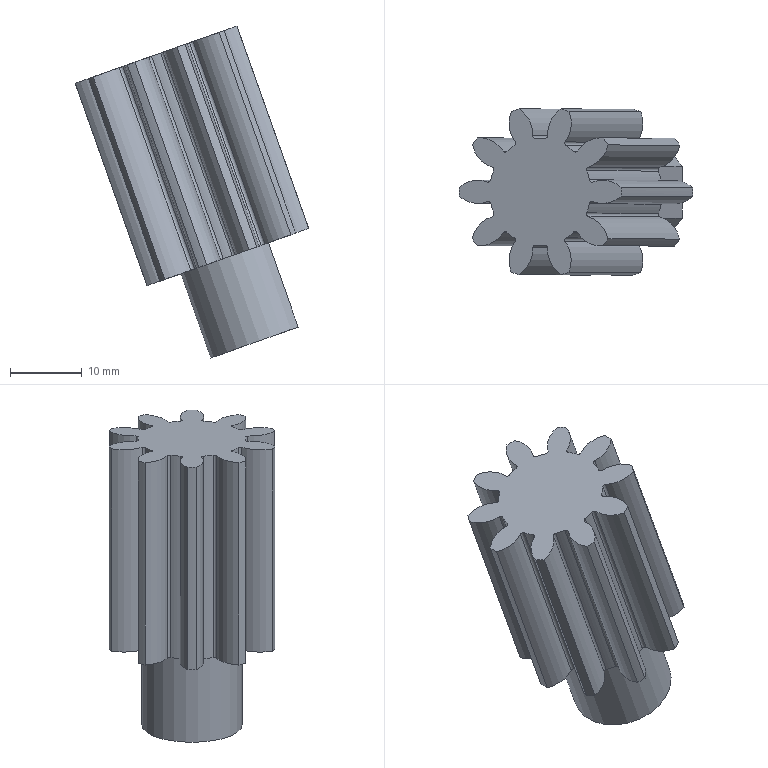Part | STEP file | GEAR1-3_id414_x_t | 1 solid | 65 faces | box 32.638 x 23.177 x 46.405 mm | volume 10951 mm3 | cylinder 61 | plane 4 | commonest cylinder face diameters 0.8 x20 8.393 x20 15 x10 24 x10 14 x1